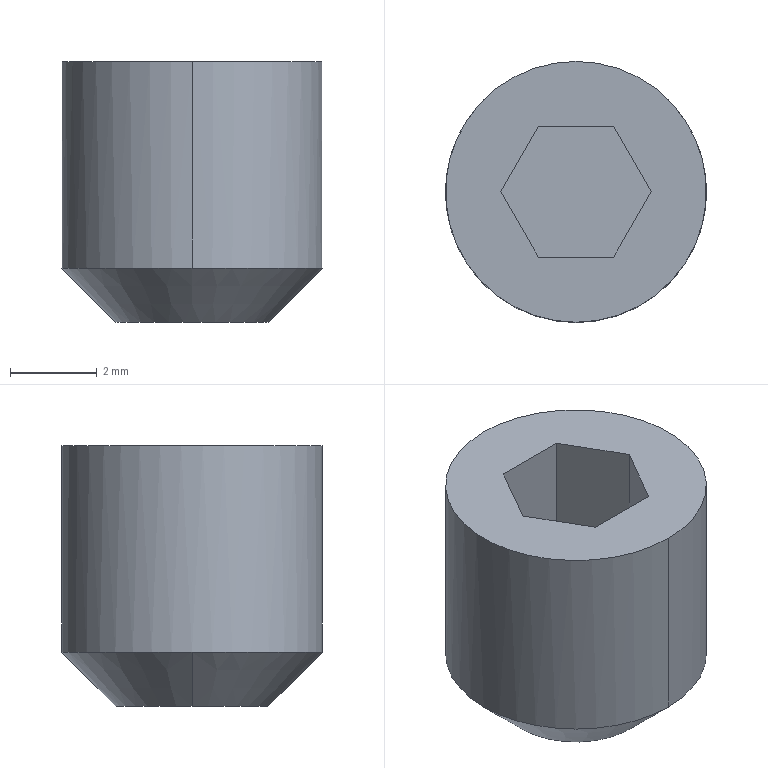Part | STEP file | Microwave Drying Flat Conveyor-inafag_ucfl204_62o9y6gnj3059x015y4y3bh4_12 | 1 solid | 14 faces | box 6 x 6 x 6 mm | volume 135.214 mm3 | plane 8 | cone 4 | cylinder 2 | commonest cylinder face diameters 6 x2
STEP:
#1=CARTESIAN_POINT('',(31.3,0.,11.25));
#2=VERTEX_POINT('',#1);
#3=CARTESIAN_POINT('',(28.3,3.,11.25));
#4=VERTEX_POINT('',#3);
#5=CARTESIAN_POINT('',(28.3,0.,11.25));
#6=DIRECTION('',(0.,0.,1.));
#7=DIRECTION('',(0.,-1.,0.));
#8=AXIS2_PLACEMENT_3D('',#5,#6,#7);
#9=CIRCLE('',#8,3.);
#10=EDGE_CURVE('',#2,#4,#9,.T.);
#11=ORIENTED_EDGE('',*,*,#10,.T.);
#12=CARTESIAN_POINT('',(28.3,3.,16.));
#13=VERTEX_POINT('',#12);
#14=CARTESIAN_POINT('',(28.3,3.,13.625));
#15=DIRECTION('',(0.,0.,1.));
#16=VECTOR('',#15,1000.);
#17=LINE('',#14,#16);
#18=EDGE_CURVE('',#4,#13,#17,.T.);
#19=ORIENTED_EDGE('',*,*,#18,.T.);
#20=CARTESIAN_POINT('',(28.3,-3.,16.));
#21=VERTEX_POINT('',#20);
#22=CARTESIAN_POINT('',(28.3,0.,16.));
#23=DIRECTION('',(0.,0.,-1.));
#24=DIRECTION('',(0.,-1.,0.));
#25=AXIS2_PLACEMENT_3D('',#22,#23,#24);
#26=CIRCLE('',#25,3.);
#27=EDGE_CURVE('',#13,#21,#26,.T.);
#28=ORIENTED_EDGE('',*,*,#27,.T.);
#29=CARTESIAN_POINT('',(28.3,-3.,11.25));
#30=VERTEX_POINT('',#29);
#31=CARTESIAN_POINT('',(28.3,-3.,13.625));
#32=DIRECTION('',(0.,0.,1.));
#33=VECTOR('',#32,1000.);
#34=LINE('',#31,#33);
#35=EDGE_CURVE('',#30,#21,#34,.T.);
#36=ORIENTED_EDGE('',*,*,#35,.F.);
#37=CARTESIAN_POINT('',(28.3,0.,11.25));
#38=DIRECTION('',(0.,0.,1.));
#39=DIRECTION('',(0.,-1.,0.));
#40=AXIS2_PLACEMENT_3D('',#37,#38,#39);
#41=CIRCLE('',#40,3.);
#42=EDGE_CURVE('',#30,#2,#41,.T.);
#43=ORIENTED_EDGE('',*,*,#42,.T.);
#44=EDGE_LOOP('',(#11,#19,#28,#36,#43));
#45=FACE_OUTER_BOUND('',#44,.T.);
#46=CARTESIAN_POINT('',(28.3,0.,13.625));
#47=DIRECTION('',(0.,0.,1.));
#48=DIRECTION('',(0.,-1.,0.));
#49=AXIS2_PLACEMENT_3D('',#46,#47,#48);
#50=CYLINDRICAL_SURFACE('',#49,3.);
#51=ADVANCED_FACE('',(#45),#50,.T.);
#52=CARTESIAN_POINT('',(30.05,0.,10.));
#53=VERTEX_POINT('',#52);
#54=CARTESIAN_POINT('',(26.55,0.,10.));
#55=VERTEX_POINT('',#54);
#56=CARTESIAN_POINT('',(28.3,0.,10.));
#57=DIRECTION('',(0.,0.,1.));
#58=DIRECTION('',(1.,0.,0.));
#59=AXIS2_PLACEMENT_3D('',#56,#57,#58);
#60=CIRCLE('',#59,1.75);
#61=EDGE_CURVE('',#53,#55,#60,.T.);
#62=ORIENTED_EDGE('',*,*,#61,.T.);
#63=CARTESIAN_POINT('',(25.3,0.,11.25));
#64=VERTEX_POINT('',#63);
#65=CARTESIAN_POINT('',(25.3,0.,11.25));
#66=DIRECTION('',(-0.7071,0.,0.7071));
#67=VECTOR('',#66,1000.);
#68=LINE('',#65,#67);
#69=EDGE_CURVE('',#55,#64,#68,.T.);
#70=ORIENTED_EDGE('',*,*,#69,.T.);
#71=CARTESIAN_POINT('',(28.3,0.,11.25));
#72=DIRECTION('',(0.,0.,1.));
#73=DIRECTION('',(0.,-1.,0.));
#74=AXIS2_PLACEMENT_3D('',#71,#72,#73);
#75=CIRCLE('',#74,3.);
#76=EDGE_CURVE('',#4,#64,#75,.T.);
#77=ORIENTED_EDGE('',*,*,#76,.F.);
#78=ORIENTED_EDGE('',*,*,#10,.F.);
#79=CARTESIAN_POINT('',(31.3,0.,11.25));
#80=DIRECTION('',(0.7071,0.,0.7071));
#81=VECTOR('',#80,1000.);
#82=LINE('',#79,#81);
#83=EDGE_CURVE('',#53,#2,#82,.T.);
#84=ORIENTED_EDGE('',*,*,#83,.F.);
#85=EDGE_LOOP('',(#62,#70,#77,#78,#84));
#86=FACE_OUTER_BOUND('',#85,.T.);
#87=CARTESIAN_POINT('',(28.3,0.,11.25));
#88=DIRECTION('',(0.,0.,1.));
#89=DIRECTION('',(1.,0.,0.));
#90=AXIS2_PLACEMENT_3D('',#87,#88,#89);
#91=CONICAL_SURFACE('',#90,3.,0.7854);
#92=ADVANCED_FACE('',(#86),#91,.T.);
#93=CARTESIAN_POINT('',(28.3,0.,11.01));
#94=VERTEX_POINT('',#93);
#95=CARTESIAN_POINT('',(28.3,0.,11.01));
#96=DIRECTION('',(-0.866,0.,-0.5));
#97=VECTOR('',#96,1000.);
#98=LINE('',#95,#97);
#99=EDGE_CURVE('',#94,#55,#98,.T.);
#100=ORIENTED_EDGE('',*,*,#99,.F.);
#101=CARTESIAN_POINT('',(28.3,0.,11.01));
#102=DIRECTION('',(0.866,0.,-0.5));
#103=VECTOR('',#102,1000.);
#104=LINE('',#101,#103);
#105=EDGE_CURVE('',#94,#53,#104,.T.);
#106=ORIENTED_EDGE('',*,*,#105,.T.);
#107=CARTESIAN_POINT('',(28.3,0.,10.));
#108=DIRECTION('',(0.,0.,1.));
#109=DIRECTION('',(1.,0.,0.));
#110=AXIS2_PLACEMENT_3D('',#107,#108,#109);
#111=CIRCLE('',#110,1.75);
#112=EDGE_CURVE('',#55,#53,#111,.T.);
#113=ORIENTED_EDGE('',*,*,#112,.F.);
#114=EDGE_LOOP('',(#100,#106,#113));
#115=FACE_OUTER_BOUND('',#114,.T.);
#116=CARTESIAN_POINT('',(28.3,0.,-988.99));
#117=DIRECTION('',(0.,0.,-1.));
#118=DIRECTION('',(-1.,0.,0.));
#119=AXIS2_PLACEMENT_3D('',#116,#117,#118);
#120=CONICAL_SURFACE('',#119,1732.051,1.047);
#121=ADVANCED_FACE('',(#115),#120,.F.);
#122=ORIENTED_EDGE('',*,*,#18,.F.);
#123=ORIENTED_EDGE('',*,*,#76,.T.);
#124=CARTESIAN_POINT('',(28.3,0.,11.25));
#125=DIRECTION('',(0.,0.,1.));
#126=DIRECTION('',(0.,-1.,0.));
#127=AXIS2_PLACEMENT_3D('',#124,#125,#126);
#128=CIRCLE('',#127,3.);
#129=EDGE_CURVE('',#64,#30,#128,.T.);
#130=ORIENTED_EDGE('',*,*,#129,.T.);
#131=ORIENTED_EDGE('',*,*,#35,.T.);
#132=CARTESIAN_POINT('',(28.3,0.,16.));
#133=DIRECTION('',(0.,0.,-1.));
#134=DIRECTION('',(0.,-1.,0.));
#135=AXIS2_PLACEMENT_3D('',#132,#133,#134);
#136=CIRCLE('',#135,3.);
#137=EDGE_CURVE('',#21,#13,#136,.T.);
#138=ORIENTED_EDGE('',*,*,#137,.T.);
#139=EDGE_LOOP('',(#122,#123,#130,#131,#138));
#140=FACE_OUTER_BOUND('',#139,.T.);
#141=CARTESIAN_POINT('',(28.3,0.,13.625));
#142=DIRECTION('',(0.,0.,1.));
#143=DIRECTION('',(0.,-1.,0.));
#144=AXIS2_PLACEMENT_3D('',#141,#142,#143);
#145=CYLINDRICAL_SURFACE('',#144,3.);
#146=ADVANCED_FACE('',(#140),#145,.T.);
#147=ORIENTED_EDGE('',*,*,#137,.F.);
#148=ORIENTED_EDGE('',*,*,#27,.F.);
#149=EDGE_LOOP('',(#147,#148));
#150=FACE_OUTER_BOUND('',#149,.T.);
#151=CARTESIAN_POINT('',(27.434,-1.5,16.));
#152=VERTEX_POINT('',#151);
#153=CARTESIAN_POINT('',(26.568,0.,16.));
#154=VERTEX_POINT('',#153);
#155=CARTESIAN_POINT('',(27.001,-0.75,16.));
#156=DIRECTION('',(-0.5,0.866,0.));
#157=VECTOR('',#156,1000.);
#158=LINE('',#155,#157);
#159=EDGE_CURVE('',#152,#154,#158,.T.);
#160=ORIENTED_EDGE('',*,*,#159,.T.);
#161=CARTESIAN_POINT('',(27.434,1.5,16.));
#162=VERTEX_POINT('',#161);
#163=CARTESIAN_POINT('',(26.568,0.,16.));
#164=DIRECTION('',(0.5,0.866,0.));
#165=VECTOR('',#164,1000.);
#166=LINE('',#163,#165);
#167=EDGE_CURVE('',#154,#162,#166,.T.);
#168=ORIENTED_EDGE('',*,*,#167,.T.);
#169=CARTESIAN_POINT('',(29.166,1.5,16.));
#170=VERTEX_POINT('',#169);
#171=CARTESIAN_POINT('',(28.733,1.5,16.));
#172=DIRECTION('',(1.,0.,0.));
#173=VECTOR('',#172,1000.);
#174=LINE('',#171,#173);
#175=EDGE_CURVE('',#162,#170,#174,.T.);
#176=ORIENTED_EDGE('',*,*,#175,.T.);
#177=CARTESIAN_POINT('',(30.032,0.,16.));
#178=VERTEX_POINT('',#177);
#179=CARTESIAN_POINT('',(29.599,0.75,16.));
#180=DIRECTION('',(0.5,-0.866,0.));
#181=VECTOR('',#180,1000.);
#182=LINE('',#179,#181);
#183=EDGE_CURVE('',#170,#178,#182,.T.);
#184=ORIENTED_EDGE('',*,*,#183,.T.);
#185=CARTESIAN_POINT('',(29.166,-1.5,16.));
#186=VERTEX_POINT('',#185);
#187=CARTESIAN_POINT('',(29.599,-0.75,16.));
#188=DIRECTION('',(-0.5,-0.866,0.));
#189=VECTOR('',#188,1000.);
#190=LINE('',#187,#189);
#191=EDGE_CURVE('',#178,#186,#190,.T.);
#192=ORIENTED_EDGE('',*,*,#191,.T.);
#193=CARTESIAN_POINT('',(28.3,-1.5,16.));
#194=DIRECTION('',(-1.,0.,0.));
#195=VECTOR('',#194,1000.);
#196=LINE('',#193,#195);
#197=EDGE_CURVE('',#186,#152,#196,.T.);
#198=ORIENTED_EDGE('',*,*,#197,.T.);
#199=EDGE_LOOP('',(#160,#168,#176,#184,#192,#198));
#200=FACE_BOUND('',#199,.T.);
#201=CARTESIAN_POINT('',(29.8,0.,16.));
#202=DIRECTION('',(0.,0.,1.));
#203=DIRECTION('',(0.,-1.,0.));
#204=AXIS2_PLACEMENT_3D('',#201,#202,#203);
#205=PLANE('',#204);
#206=ADVANCED_FACE('',(#150,#200),#205,.T.);
#207=ORIENTED_EDGE('',*,*,#69,.F.);
#208=ORIENTED_EDGE('',*,*,#112,.T.);
#209=ORIENTED_EDGE('',*,*,#83,.T.);
#210=ORIENTED_EDGE('',*,*,#42,.F.);
#211=ORIENTED_EDGE('',*,*,#129,.F.);
#212=EDGE_LOOP('',(#207,#208,#209,#210,#211));
#213=FACE_OUTER_BOUND('',#212,.T.);
#214=CARTESIAN_POINT('',(28.3,0.,11.25));
#215=DIRECTION('',(0.,0.,1.));
#216=DIRECTION('',(1.,0.,0.));
#217=AXIS2_PLACEMENT_3D('',#214,#215,#216);
#218=CONICAL_SURFACE('',#217,3.,0.7854);
#219=ADVANCED_FACE('',(#213),#218,.T.);
#220=CARTESIAN_POINT('',(26.568,0.,13.625));
#221=VERTEX_POINT('',#220);
#222=CARTESIAN_POINT('',(26.568,0.,13.625));
#223=DIRECTION('',(0.,0.,1.));
#224=VECTOR('',#223,1000.);
#225=LINE('',#222,#224);
#226=EDGE_CURVE('',#221,#154,#225,.T.);
#227=ORIENTED_EDGE('',*,*,#226,.F.);
#228=CARTESIAN_POINT('',(27.434,1.5,13.625));
#229=VERTEX_POINT('',#228);
#230=CARTESIAN_POINT('',(27.001,0.75,13.625));
#231=DIRECTION('',(-0.5,-0.866,0.));
#232=VECTOR('',#231,1000.);
#233=LINE('',#230,#232);
#234=EDGE_CURVE('',#229,#221,#233,.T.);
#235=ORIENTED_EDGE('',*,*,#234,.F.);
#236=CARTESIAN_POINT('',(27.434,1.5,13.625));
#237=DIRECTION('',(0.,0.,-1.));
#238=VECTOR('',#237,1000.);
#239=LINE('',#236,#238);
#240=EDGE_CURVE('',#162,#229,#239,.T.);
#241=ORIENTED_EDGE('',*,*,#240,.F.);
#242=ORIENTED_EDGE('',*,*,#167,.F.);
#243=EDGE_LOOP('',(#227,#235,#241,#242));
#244=FACE_OUTER_BOUND('',#243,.T.);
#245=CARTESIAN_POINT('',(27.001,0.75,13.625));
#246=DIRECTION('',(-0.866,0.5,0.));
#247=DIRECTION('',(-0.5,-0.866,0.));
#248=AXIS2_PLACEMENT_3D('',#245,#246,#247);
#249=PLANE('',#248);
#250=ADVANCED_FACE('',(#244),#249,.F.);
#251=ORIENTED_EDGE('',*,*,#105,.F.);
#252=ORIENTED_EDGE('',*,*,#99,.T.);
#253=ORIENTED_EDGE('',*,*,#61,.F.);
#254=EDGE_LOOP('',(#251,#252,#253));
#255=FACE_OUTER_BOUND('',#254,.T.);
#256=CARTESIAN_POINT('',(28.3,0.,-988.99));
#257=DIRECTION('',(0.,0.,-1.));
#258=DIRECTION('',(-1.,0.,0.));
#259=AXIS2_PLACEMENT_3D('',#256,#257,#258);
#260=CONICAL_SURFACE('',#259,1732.051,1.047);
#261=ADVANCED_FACE('',(#255),#260,.F.);
#262=CARTESIAN_POINT('',(27.434,-1.5,13.625));
#263=VERTEX_POINT('',#262);
#264=CARTESIAN_POINT('',(27.434,-1.5,13.625));
#265=DIRECTION('',(0.,0.,1.));
#266=VECTOR('',#265,1000.);
#267=LINE('',#264,#266);
#268=EDGE_CURVE('',#263,#152,#267,.T.);
#269=ORIENTED_EDGE('',*,*,#268,.F.);
#270=CARTESIAN_POINT('',(27.001,-0.75,13.625));
#271=DIRECTION('',(0.5,-0.866,0.));
#272=VECTOR('',#271,1000.);
#273=LINE('',#270,#272);
#274=EDGE_CURVE('',#221,#263,#273,.T.);
#275=ORIENTED_EDGE('',*,*,#274,.F.);
#276=ORIENTED_EDGE('',*,*,#226,.T.);
#277=ORIENTED_EDGE('',*,*,#159,.F.);
#278=EDGE_LOOP('',(#269,#275,#276,#277));
#279=FACE_OUTER_BOUND('',#278,.T.);
#280=CARTESIAN_POINT('',(27.001,-0.75,13.625));
#281=DIRECTION('',(-0.866,-0.5,0.));
#282=DIRECTION('',(0.5,-0.866,0.));
#283=AXIS2_PLACEMENT_3D('',#280,#281,#282);
#284=PLANE('',#283);
#285=ADVANCED_FACE('',(#279),#284,.F.);
#286=CARTESIAN_POINT('',(29.166,-1.5,13.625));
#287=VERTEX_POINT('',#286);
#288=CARTESIAN_POINT('',(30.032,0.,13.625));
#289=VERTEX_POINT('',#288);
#290=CARTESIAN_POINT('',(29.599,-0.75,13.625));
#291=DIRECTION('',(0.5,0.866,0.));
#292=VECTOR('',#291,1000.);
#293=LINE('',#290,#292);
#294=EDGE_CURVE('',#287,#289,#293,.T.);
#295=ORIENTED_EDGE('',*,*,#294,.T.);
#296=CARTESIAN_POINT('',(29.166,1.5,13.625));
#297=VERTEX_POINT('',#296);
#298=CARTESIAN_POINT('',(29.599,0.75,13.625));
#299=DIRECTION('',(-0.5,0.866,0.));
#300=VECTOR('',#299,1000.);
#301=LINE('',#298,#300);
#302=EDGE_CURVE('',#289,#297,#301,.T.);
#303=ORIENTED_EDGE('',*,*,#302,.T.);
#304=CARTESIAN_POINT('',(28.3,1.5,13.625));
#305=DIRECTION('',(-1.,0.,0.));
#306=VECTOR('',#305,1000.);
#307=LINE('',#304,#306);
#308=EDGE_CURVE('',#297,#229,#307,.T.);
#309=ORIENTED_EDGE('',*,*,#308,.T.);
#310=ORIENTED_EDGE('',*,*,#234,.T.);
#311=ORIENTED_EDGE('',*,*,#274,.T.);
#312=CARTESIAN_POINT('',(28.3,-1.5,13.625));
#313=DIRECTION('',(1.,0.,0.));
#314=VECTOR('',#313,1000.);
#315=LINE('',#312,#314);
#316=EDGE_CURVE('',#263,#287,#315,.T.);
#317=ORIENTED_EDGE('',*,*,#316,.T.);
#318=EDGE_LOOP('',(#295,#303,#309,#310,#311,#317));
#319=FACE_OUTER_BOUND('',#318,.T.);
#320=CARTESIAN_POINT('',(28.3,0.,13.625));
#321=DIRECTION('',(0.,0.,1.));
#322=DIRECTION('',(1.,0.,0.));
#323=AXIS2_PLACEMENT_3D('',#320,#321,#322);
#324=PLANE('',#323);
#325=ADVANCED_FACE('',(#319),#324,.T.);
#326=ORIENTED_EDGE('',*,*,#240,.T.);
#327=ORIENTED_EDGE('',*,*,#308,.F.);
#328=CARTESIAN_POINT('',(29.166,1.5,13.625));
#329=DIRECTION('',(0.,0.,-1.));
#330=VECTOR('',#329,1000.);
#331=LINE('',#328,#330);
#332=EDGE_CURVE('',#170,#297,#331,.T.);
#333=ORIENTED_EDGE('',*,*,#332,.F.);
#334=ORIENTED_EDGE('',*,*,#175,.F.);
#335=EDGE_LOOP('',(#326,#327,#333,#334));
#336=FACE_OUTER_BOUND('',#335,.T.);
#337=CARTESIAN_POINT('',(28.733,1.5,13.625));
#338=DIRECTION('',(0.,1.,0.));
#339=DIRECTION('',(0.,0.,1.));
#340=AXIS2_PLACEMENT_3D('',#337,#338,#339);
#341=PLANE('',#340);
#342=ADVANCED_FACE('',(#336),#341,.F.);
#343=CARTESIAN_POINT('',(29.166,-1.5,13.625));
#344=DIRECTION('',(0.,0.,1.));
#345=VECTOR('',#344,1000.);
#346=LINE('',#343,#345);
#347=EDGE_CURVE('',#287,#186,#346,.T.);
#348=ORIENTED_EDGE('',*,*,#347,.F.);
#349=ORIENTED_EDGE('',*,*,#316,.F.);
#350=ORIENTED_EDGE('',*,*,#268,.T.);
#351=ORIENTED_EDGE('',*,*,#197,.F.);
#352=EDGE_LOOP('',(#348,#349,#350,#351));
#353=FACE_OUTER_BOUND('',#352,.T.);
#354=CARTESIAN_POINT('',(28.3,-1.5,13.625));
#355=DIRECTION('',(0.,-1.,0.));
#356=DIRECTION('',(1.,0.,0.));
#357=AXIS2_PLACEMENT_3D('',#354,#355,#356);
#358=PLANE('',#357);
#359=ADVANCED_FACE('',(#353),#358,.F.);
#360=ORIENTED_EDGE('',*,*,#332,.T.);
#361=ORIENTED_EDGE('',*,*,#302,.F.);
#362=CARTESIAN_POINT('',(30.032,0.,13.625));
#363=DIRECTION('',(0.,0.,-1.));
#364=VECTOR('',#363,1000.);
#365=LINE('',#362,#364);
#366=EDGE_CURVE('',#178,#289,#365,.T.);
#367=ORIENTED_EDGE('',*,*,#366,.F.);
#368=ORIENTED_EDGE('',*,*,#183,.F.);
#369=EDGE_LOOP('',(#360,#361,#367,#368));
#370=FACE_OUTER_BOUND('',#369,.T.);
#371=CARTESIAN_POINT('',(29.599,0.75,13.625));
#372=DIRECTION('',(0.866,0.5,0.));
#373=DIRECTION('',(-0.5,0.866,0.));
#374=AXIS2_PLACEMENT_3D('',#371,#372,#373);
#375=PLANE('',#374);
#376=ADVANCED_FACE('',(#370),#375,.F.);
#377=ORIENTED_EDGE('',*,*,#366,.T.);
#378=ORIENTED_EDGE('',*,*,#294,.F.);
#379=ORIENTED_EDGE('',*,*,#347,.T.);
#380=ORIENTED_EDGE('',*,*,#191,.F.);
#381=EDGE_LOOP('',(#377,#378,#379,#380));
#382=FACE_OUTER_BOUND('',#381,.T.);
#383=CARTESIAN_POINT('',(29.599,-0.75,13.625));
#384=DIRECTION('',(0.866,-0.5,0.));
#385=DIRECTION('',(0.5,0.866,0.));
#386=AXIS2_PLACEMENT_3D('',#383,#384,#385);
#387=PLANE('',#386);
#388=ADVANCED_FACE('',(#382),#387,.F.);
#389=CLOSED_SHELL('',(#51,#92,#121,#146,#206,#219,#250,#261,#285,#325,#342,#359,#376,#388));
#390=MANIFOLD_SOLID_BREP('',#389);
#391=CARTESIAN_POINT('',(0.,0.,0.));
#392=DIRECTION('',(0.,0.,1.));
#393=DIRECTION('',(1.,0.,0.));
#394=AXIS2_PLACEMENT_3D('',#391,#392,#393);
#395=(LENGTH_UNIT()NAMED_UNIT(*)SI_UNIT(.MILLI.,.METRE.));
#396=UNCERTAINTY_MEASURE_WITH_UNIT(LENGTH_MEASURE(0.00001),#395,'','');
#397=(NAMED_UNIT(*)PLANE_ANGLE_UNIT()SI_UNIT($,.RADIAN.));
#398=(NAMED_UNIT(*)SI_UNIT($,.STERADIAN.)SOLID_ANGLE_UNIT());
#399=(GEOMETRIC_REPRESENTATION_CONTEXT(3)GLOBAL_UNCERTAINTY_ASSIGNED_CONTEXT((#396))GLOBAL_UNIT_ASSIGNED_CONTEXT((#395,#397,#398))REPRESENTATION_CONTEXT('',''));
#400=ADVANCED_BREP_SHAPE_REPRESENTATION('',(#390,#394),#399);